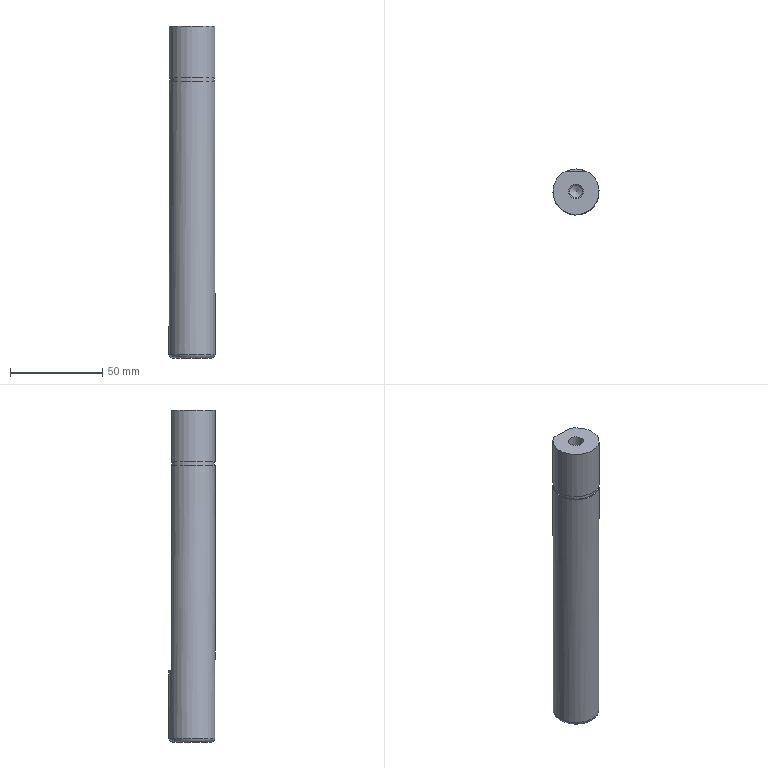Part | NX | features 18 2 | 1 solid | 14 faces | box 25 x 25 x 180 mm | volume 85420 mm3 | plane 6 | cylinder 5 | cone 2 | torus 1 | commonest cylinder face diameters 25 x2 6.8 x1 8 x1 24 x1
STEP:
#1=CARTESIAN_POINT('',(3146.937,451.,-170.));
#2=VERTEX_POINT('',#1);
#3=CARTESIAN_POINT('',(3135.063,451.,-170.));
#4=VERTEX_POINT('',#3);
#5=CARTESIAN_POINT('',(3141.,440.,-170.));
#6=DIRECTION('',(0.,0.,1.));
#7=DIRECTION('',(1.,0.,0.));
#8=AXIS2_PLACEMENT_3D('',#5,#6,#7);
#9=CIRCLE('',#8,12.5);
#10=EDGE_CURVE('',#2,#4,#9,.T.);
#11=ORIENTED_EDGE('',*,*,#10,.F.);
#12=CARTESIAN_POINT('',(3146.937,451.,-58.5));
#13=VERTEX_POINT('',#12);
#14=CARTESIAN_POINT('',(3146.937,451.,-118.5));
#15=DIRECTION('',(0.,0.,-1.));
#16=VECTOR('',#15,1000.);
#17=LINE('',#14,#16);
#18=EDGE_CURVE('',#13,#2,#17,.T.);
#19=ORIENTED_EDGE('',*,*,#18,.F.);
#20=CARTESIAN_POINT('',(3135.063,451.,-58.5));
#21=VERTEX_POINT('',#20);
#22=CARTESIAN_POINT('',(3141.,440.,-58.5));
#23=DIRECTION('',(0.,0.,1.));
#24=DIRECTION('',(-1.,0.,0.));
#25=AXIS2_PLACEMENT_3D('',#22,#23,#24);
#26=CIRCLE('',#25,12.5);
#27=EDGE_CURVE('',#21,#13,#26,.T.);
#28=ORIENTED_EDGE('',*,*,#27,.F.);
#29=CARTESIAN_POINT('',(3135.063,451.,-118.5));
#30=DIRECTION('',(0.,0.,1.));
#31=VECTOR('',#30,1000.);
#32=LINE('',#29,#31);
#33=EDGE_CURVE('',#4,#21,#32,.T.);
#34=ORIENTED_EDGE('',*,*,#33,.F.);
#35=EDGE_LOOP('',(#11,#19,#28,#34));
#36=FACE_BOUND('',#35,.T.);
#37=CARTESIAN_POINT('',(3128.5,440.,-206.5));
#38=VERTEX_POINT('',#37);
#39=CARTESIAN_POINT('',(3141.,440.,-206.5));
#40=DIRECTION('',(0.,0.,1.));
#41=DIRECTION('',(-1.,0.,0.));
#42=AXIS2_PLACEMENT_3D('',#39,#40,#41);
#43=CIRCLE('',#42,12.5);
#44=EDGE_CURVE('',#38,#38,#43,.T.);
#45=ORIENTED_EDGE('',*,*,#44,.T.);
#46=EDGE_LOOP('',(#45));
#47=FACE_BOUND('',#46,.T.);
#48=CARTESIAN_POINT('',(3141.,440.,-118.5));
#49=DIRECTION('',(0.,0.,-1.));
#50=DIRECTION('',(0.008727,1.,0.));
#51=AXIS2_PLACEMENT_3D('',#48,#49,#50);
#52=CYLINDRICAL_SURFACE('',#51,12.5);
#53=ADVANCED_FACE('',(#36,#47),#52,.T.);
#54=CARTESIAN_POINT('',(3130.5,440.,-208.5));
#55=VERTEX_POINT('',#54);
#56=CARTESIAN_POINT('',(3141.,440.,-208.5));
#57=DIRECTION('',(0.,0.,-1.));
#58=DIRECTION('',(-1.,0.,0.));
#59=AXIS2_PLACEMENT_3D('',#56,#57,#58);
#60=CIRCLE('',#59,10.5);
#61=EDGE_CURVE('',#55,#55,#60,.T.);
#62=ORIENTED_EDGE('',*,*,#61,.F.);
#63=EDGE_LOOP('',(#62));
#64=FACE_BOUND('',#63,.T.);
#65=ORIENTED_EDGE('',*,*,#44,.F.);
#66=EDGE_LOOP('',(#65));
#67=FACE_BOUND('',#66,.T.);
#68=CARTESIAN_POINT('',(3141.,440.,-206.5));
#69=DIRECTION('',(0.,0.,-1.));
#70=DIRECTION('',(-1.,0.,0.));
#71=AXIS2_PLACEMENT_3D('',#68,#69,#70);
#72=TOROIDAL_SURFACE('',#71,10.5,2.);
#73=ADVANCED_FACE('',(#64,#67),#72,.T.);
#74=CARTESIAN_POINT('',(3145.796,451.,-58.5));
#75=VERTEX_POINT('',#74);
#76=CARTESIAN_POINT('',(3136.204,451.,-58.5));
#77=VERTEX_POINT('',#76);
#78=CARTESIAN_POINT('',(3141.,440.,-58.5));
#79=DIRECTION('',(0.,0.,-1.));
#80=DIRECTION('',(1.,0.,0.));
#81=AXIS2_PLACEMENT_3D('',#78,#79,#80);
#82=CIRCLE('',#81,12.);
#83=EDGE_CURVE('',#75,#77,#82,.T.);
#84=ORIENTED_EDGE('',*,*,#83,.F.);
#85=CARTESIAN_POINT('',(3145.796,451.,-56.5));
#86=VERTEX_POINT('',#85);
#87=CARTESIAN_POINT('',(3145.796,451.,-57.5));
#88=DIRECTION('',(0.,0.,-1.));
#89=VECTOR('',#88,1000.);
#90=LINE('',#87,#89);
#91=EDGE_CURVE('',#86,#75,#90,.T.);
#92=ORIENTED_EDGE('',*,*,#91,.F.);
#93=CARTESIAN_POINT('',(3136.204,451.,-56.5));
#94=VERTEX_POINT('',#93);
#95=CARTESIAN_POINT('',(3141.,440.,-56.5));
#96=DIRECTION('',(0.,0.,1.));
#97=DIRECTION('',(1.,0.,0.));
#98=AXIS2_PLACEMENT_3D('',#95,#96,#97);
#99=CIRCLE('',#98,12.);
#100=EDGE_CURVE('',#94,#86,#99,.T.);
#101=ORIENTED_EDGE('',*,*,#100,.F.);
#102=CARTESIAN_POINT('',(3136.204,451.,-57.5));
#103=DIRECTION('',(0.,0.,1.));
#104=VECTOR('',#103,1000.);
#105=LINE('',#102,#104);
#106=EDGE_CURVE('',#77,#94,#105,.T.);
#107=ORIENTED_EDGE('',*,*,#106,.F.);
#108=EDGE_LOOP('',(#84,#92,#101,#107));
#109=FACE_BOUND('',#108,.T.);
#110=CARTESIAN_POINT('',(3141.,440.,-57.5));
#111=DIRECTION('',(0.,0.,-1.));
#112=DIRECTION('',(1.,0.,0.));
#113=AXIS2_PLACEMENT_3D('',#110,#111,#112);
#114=CYLINDRICAL_SURFACE('',#113,12.);
#115=ADVANCED_FACE('',(#109),#114,.T.);
#116=CARTESIAN_POINT('',(3135.063,451.,-56.5));
#117=VERTEX_POINT('',#116);
#118=CARTESIAN_POINT('',(3157.25,451.,-56.5));
#119=DIRECTION('',(1.,0.,0.));
#120=VECTOR('',#119,1000.);
#121=LINE('',#118,#120);
#122=EDGE_CURVE('',#117,#94,#121,.T.);
#123=ORIENTED_EDGE('',*,*,#122,.T.);
#124=ORIENTED_EDGE('',*,*,#100,.T.);
#125=CARTESIAN_POINT('',(3146.937,451.,-56.5));
#126=VERTEX_POINT('',#125);
#127=CARTESIAN_POINT('',(3157.25,451.,-56.5));
#128=DIRECTION('',(1.,0.,0.));
#129=VECTOR('',#128,1000.);
#130=LINE('',#127,#129);
#131=EDGE_CURVE('',#86,#126,#130,.T.);
#132=ORIENTED_EDGE('',*,*,#131,.T.);
#133=CARTESIAN_POINT('',(3141.,440.,-56.5));
#134=DIRECTION('',(0.,0.,-1.));
#135=DIRECTION('',(1.,0.,0.));
#136=AXIS2_PLACEMENT_3D('',#133,#134,#135);
#137=CIRCLE('',#136,12.5);
#138=EDGE_CURVE('',#126,#117,#137,.T.);
#139=ORIENTED_EDGE('',*,*,#138,.T.);
#140=EDGE_LOOP('',(#123,#124,#132,#139));
#141=FACE_BOUND('',#140,.T.);
#142=CARTESIAN_POINT('',(3157.25,414.019,-56.5));
#143=DIRECTION('',(0.,0.,1.));
#144=DIRECTION('',(-1.,0.,0.));
#145=AXIS2_PLACEMENT_3D('',#142,#143,#144);
#146=PLANE('',#145);
#147=ADVANCED_FACE('',(#141),#146,.F.);
#148=CARTESIAN_POINT('',(3112.25,451.,-58.5));
#149=DIRECTION('',(-1.,0.,0.));
#150=VECTOR('',#149,1000.);
#151=LINE('',#148,#150);
#152=EDGE_CURVE('',#13,#75,#151,.T.);
#153=ORIENTED_EDGE('',*,*,#152,.T.);
#154=ORIENTED_EDGE('',*,*,#83,.T.);
#155=CARTESIAN_POINT('',(3112.25,451.,-58.5));
#156=DIRECTION('',(-1.,0.,0.));
#157=VECTOR('',#156,1000.);
#158=LINE('',#155,#157);
#159=EDGE_CURVE('',#77,#21,#158,.T.);
#160=ORIENTED_EDGE('',*,*,#159,.T.);
#161=ORIENTED_EDGE('',*,*,#27,.T.);
#162=EDGE_LOOP('',(#153,#154,#160,#161));
#163=FACE_BOUND('',#162,.T.);
#164=CARTESIAN_POINT('',(3112.25,414.019,-58.5));
#165=DIRECTION('',(0.,0.,-1.));
#166=DIRECTION('',(1.,0.,0.));
#167=AXIS2_PLACEMENT_3D('',#164,#165,#166);
#168=PLANE('',#167);
#169=ADVANCED_FACE('',(#163),#168,.F.);
#170=ORIENTED_EDGE('',*,*,#138,.F.);
#171=CARTESIAN_POINT('',(3146.937,451.,-28.5));
#172=VERTEX_POINT('',#171);
#173=CARTESIAN_POINT('',(3146.937,451.,-118.5));
#174=DIRECTION('',(0.,0.,-1.));
#175=VECTOR('',#174,1000.);
#176=LINE('',#173,#175);
#177=EDGE_CURVE('',#172,#126,#176,.T.);
#178=ORIENTED_EDGE('',*,*,#177,.F.);
#179=CARTESIAN_POINT('',(3135.063,451.,-28.5));
#180=VERTEX_POINT('',#179);
#181=CARTESIAN_POINT('',(3141.,440.,-28.5));
#182=DIRECTION('',(0.,0.,-1.));
#183=DIRECTION('',(1.,0.,0.));
#184=AXIS2_PLACEMENT_3D('',#181,#182,#183);
#185=CIRCLE('',#184,12.5);
#186=EDGE_CURVE('',#172,#180,#185,.T.);
#187=ORIENTED_EDGE('',*,*,#186,.T.);
#188=CARTESIAN_POINT('',(3135.063,451.,-118.5));
#189=DIRECTION('',(0.,0.,1.));
#190=VECTOR('',#189,1000.);
#191=LINE('',#188,#190);
#192=EDGE_CURVE('',#117,#180,#191,.T.);
#193=ORIENTED_EDGE('',*,*,#192,.F.);
#194=EDGE_LOOP('',(#170,#178,#187,#193));
#195=FACE_BOUND('',#194,.T.);
#196=CARTESIAN_POINT('',(3141.,440.,-118.5));
#197=DIRECTION('',(0.,0.,-1.));
#198=DIRECTION('',(1.,0.,0.));
#199=AXIS2_PLACEMENT_3D('',#196,#197,#198);
#200=CYLINDRICAL_SURFACE('',#199,12.5);
#201=ADVANCED_FACE('',(#195),#200,.T.);
#202=CARTESIAN_POINT('',(3145.,440.,-28.5));
#203=VERTEX_POINT('',#202);
#204=CARTESIAN_POINT('',(3141.,440.,-28.5));
#205=DIRECTION('',(0.,0.,1.));
#206=DIRECTION('',(1.,0.,0.));
#207=AXIS2_PLACEMENT_3D('',#204,#205,#206);
#208=CIRCLE('',#207,4.);
#209=EDGE_CURVE('',#203,#203,#208,.T.);
#210=ORIENTED_EDGE('',*,*,#209,.F.);
#211=EDGE_LOOP('',(#210));
#212=FACE_BOUND('',#211,.T.);
#213=ORIENTED_EDGE('',*,*,#186,.F.);
#214=CARTESIAN_POINT('',(3157.25,451.,-28.5));
#215=DIRECTION('',(-1.,0.,0.));
#216=VECTOR('',#215,1000.);
#217=LINE('',#214,#216);
#218=EDGE_CURVE('',#172,#180,#217,.T.);
#219=ORIENTED_EDGE('',*,*,#218,.T.);
#220=EDGE_LOOP('',(#213,#219));
#221=FACE_BOUND('',#220,.T.);
#222=CARTESIAN_POINT('',(3157.25,414.019,-28.5));
#223=DIRECTION('',(0.,0.,1.));
#224=DIRECTION('',(-1.,0.,0.));
#225=AXIS2_PLACEMENT_3D('',#222,#223,#224);
#226=PLANE('',#225);
#227=ADVANCED_FACE('',(#212,#221),#226,.T.);
#228=ORIENTED_EDGE('',*,*,#61,.T.);
#229=EDGE_LOOP('',(#228));
#230=FACE_BOUND('',#229,.T.);
#231=CARTESIAN_POINT('',(3116.85,418.176,-208.5));
#232=DIRECTION('',(0.,0.,-1.));
#233=DIRECTION('',(1.,0.,0.));
#234=AXIS2_PLACEMENT_3D('',#231,#232,#233);
#235=PLANE('',#234);
#236=ADVANCED_FACE('',(#230),#235,.T.);
#237=CARTESIAN_POINT('',(3144.4,440.,-50.5));
#238=VERTEX_POINT('',#237);
#239=CARTESIAN_POINT('',(3141.,440.,-50.5));
#240=DIRECTION('',(0.,0.,1.));
#241=DIRECTION('',(1.,0.,0.));
#242=AXIS2_PLACEMENT_3D('',#239,#240,#241);
#243=CIRCLE('',#242,3.4);
#244=EDGE_CURVE('',#238,#238,#243,.T.);
#245=ORIENTED_EDGE('',*,*,#244,.T.);
#246=EDGE_LOOP('',(#245));
#247=FACE_BOUND('',#246,.T.);
#248=CARTESIAN_POINT('',(3141.,440.,-52.463));
#249=VERTEX_POINT('',#248);
#250=VERTEX_LOOP('',#249);
#251=FACE_BOUND('',#250,.T.);
#252=CARTESIAN_POINT('',(3141.,440.,-49.687));
#253=DIRECTION('',(0.,0.,1.));
#254=DIRECTION('',(1.,0.,0.));
#255=AXIS2_PLACEMENT_3D('',#252,#253,#254);
#256=CONICAL_SURFACE('',#255,4.808,1.047);
#257=ADVANCED_FACE('',(#247,#251),#256,.F.);
#258=ORIENTED_EDGE('',*,*,#244,.F.);
#259=EDGE_LOOP('',(#258));
#260=FACE_BOUND('',#259,.T.);
#261=CARTESIAN_POINT('',(3144.4,440.,-49.));
#262=VERTEX_POINT('',#261);
#263=CARTESIAN_POINT('',(3141.,440.,-49.));
#264=DIRECTION('',(0.,0.,1.));
#265=DIRECTION('',(1.,0.,0.));
#266=AXIS2_PLACEMENT_3D('',#263,#264,#265);
#267=CIRCLE('',#266,3.4);
#268=EDGE_CURVE('',#262,#262,#267,.T.);
#269=ORIENTED_EDGE('',*,*,#268,.T.);
#270=EDGE_LOOP('',(#269));
#271=FACE_BOUND('',#270,.T.);
#272=CARTESIAN_POINT('',(3141.,440.,-49.75));
#273=DIRECTION('',(0.,0.,-1.));
#274=DIRECTION('',(1.,0.,0.));
#275=AXIS2_PLACEMENT_3D('',#272,#273,#274);
#276=CYLINDRICAL_SURFACE('',#275,3.4);
#277=ADVANCED_FACE('',(#260,#271),#276,.F.);
#278=CARTESIAN_POINT('',(3145.,440.,-48.5));
#279=VERTEX_POINT('',#278);
#280=CARTESIAN_POINT('',(3141.,440.,-48.5));
#281=DIRECTION('',(0.,0.,1.));
#282=DIRECTION('',(1.,0.,0.));
#283=AXIS2_PLACEMENT_3D('',#280,#281,#282);
#284=CIRCLE('',#283,4.);
#285=EDGE_CURVE('',#279,#279,#284,.T.);
#286=ORIENTED_EDGE('',*,*,#285,.T.);
#287=EDGE_LOOP('',(#286));
#288=FACE_BOUND('',#287,.T.);
#289=ORIENTED_EDGE('',*,*,#268,.F.);
#290=EDGE_LOOP('',(#289));
#291=FACE_BOUND('',#290,.T.);
#292=CARTESIAN_POINT('',(3141.,440.,-47.119));
#293=DIRECTION('',(0.,0.,1.));
#294=DIRECTION('',(1.,0.,0.));
#295=AXIS2_PLACEMENT_3D('',#292,#293,#294);
#296=CONICAL_SURFACE('',#295,5.657,0.8761);
#297=ADVANCED_FACE('',(#288,#291),#296,.F.);
#298=ORIENTED_EDGE('',*,*,#285,.F.);
#299=EDGE_LOOP('',(#298));
#300=FACE_BOUND('',#299,.T.);
#301=ORIENTED_EDGE('',*,*,#209,.T.);
#302=EDGE_LOOP('',(#301));
#303=FACE_BOUND('',#302,.T.);
#304=CARTESIAN_POINT('',(3141.,440.,-38.5));
#305=DIRECTION('',(0.,0.,-1.));
#306=DIRECTION('',(1.,0.,0.));
#307=AXIS2_PLACEMENT_3D('',#304,#305,#306);
#308=CYLINDRICAL_SURFACE('',#307,4.);
#309=ADVANCED_FACE('',(#300,#303),#308,.F.);
#310=CARTESIAN_POINT('',(3141.,451.,-170.));
#311=DIRECTION('',(-1.,0.,0.));
#312=VECTOR('',#311,1000.);
#313=LINE('',#310,#312);
#314=EDGE_CURVE('',#2,#4,#313,.T.);
#315=ORIENTED_EDGE('',*,*,#314,.T.);
#316=ORIENTED_EDGE('',*,*,#33,.T.);
#317=ORIENTED_EDGE('',*,*,#159,.F.);
#318=ORIENTED_EDGE('',*,*,#106,.T.);
#319=ORIENTED_EDGE('',*,*,#122,.F.);
#320=ORIENTED_EDGE('',*,*,#192,.T.);
#321=ORIENTED_EDGE('',*,*,#218,.F.);
#322=ORIENTED_EDGE('',*,*,#177,.T.);
#323=ORIENTED_EDGE('',*,*,#131,.F.);
#324=ORIENTED_EDGE('',*,*,#91,.T.);
#325=ORIENTED_EDGE('',*,*,#152,.F.);
#326=ORIENTED_EDGE('',*,*,#18,.T.);
#327=EDGE_LOOP('',(#315,#316,#317,#318,#319,#320,#321,#322,#323,#324,#325,#326));
#328=FACE_BOUND('',#327,.T.);
#329=CARTESIAN_POINT('',(3141.,451.,-63.5));
#330=DIRECTION('',(0.,1.,0.));
#331=DIRECTION('',(0.,0.,-1.));
#332=AXIS2_PLACEMENT_3D('',#329,#330,#331);
#333=PLANE('',#332);
#334=ADVANCED_FACE('',(#328),#333,.T.);
#335=ORIENTED_EDGE('',*,*,#10,.T.);
#336=ORIENTED_EDGE('',*,*,#314,.F.);
#337=EDGE_LOOP('',(#335,#336));
#338=FACE_BOUND('',#337,.T.);
#339=CARTESIAN_POINT('',(1911.,440.,-170.));
#340=DIRECTION('',(0.,0.,1.));
#341=DIRECTION('',(0.,1.,0.));
#342=AXIS2_PLACEMENT_3D('',#339,#340,#341);
#343=PLANE('',#342);
#344=ADVANCED_FACE('',(#338),#343,.T.);
#345=CLOSED_SHELL('',(#53,#73,#115,#147,#169,#201,#227,#236,#257,#277,#297,#309,#334,#344));
#346=MANIFOLD_SOLID_BREP('',#345);
#347=(LENGTH_UNIT()NAMED_UNIT(*)SI_UNIT(.MILLI.,.METRE.));
#348=UNCERTAINTY_MEASURE_WITH_UNIT(LENGTH_MEASURE(0.00001),#347,'','');
#349=(NAMED_UNIT(*)PLANE_ANGLE_UNIT()SI_UNIT($,.RADIAN.));
#350=(NAMED_UNIT(*)SI_UNIT($,.STERADIAN.)SOLID_ANGLE_UNIT());
#351=(GEOMETRIC_REPRESENTATION_CONTEXT(3)GLOBAL_UNCERTAINTY_ASSIGNED_CONTEXT((#348))GLOBAL_UNIT_ASSIGNED_CONTEXT((#347,#349,#350))REPRESENTATION_CONTEXT('',''));
#352=ADVANCED_BREP_SHAPE_REPRESENTATION('',(#346),#351);